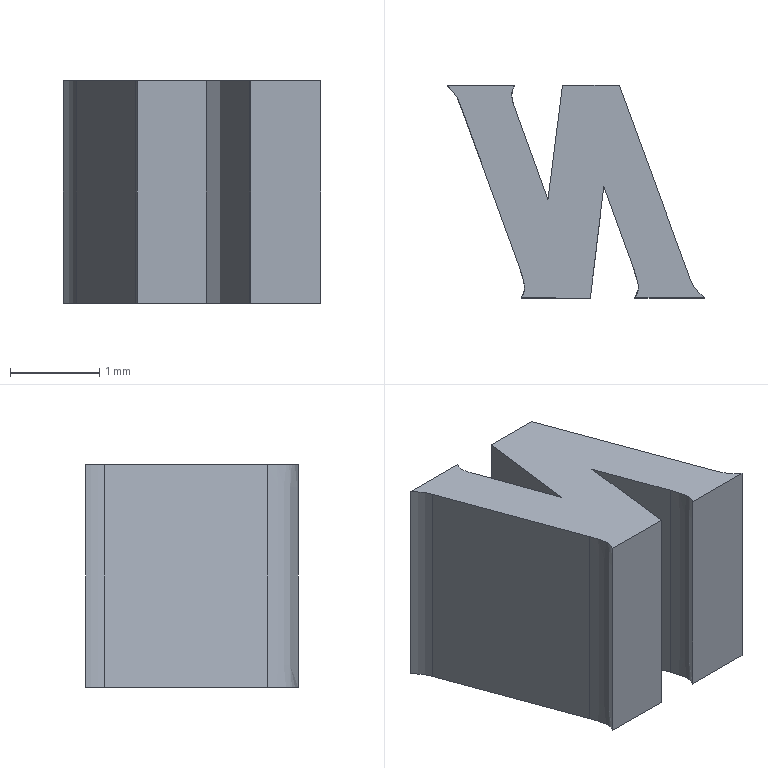Part | STEP file | lll_id1106_x_t | 1 solid | 18 faces | box 2.9 x 2.384 x 2.5 mm | volume 9.219 mm3 | plane 12 | cylinder 3 | other 3 | commonest cylinder face diameters 0.399 x1 0.832 x1 0.919 x1
STEP:
#1=CARTESIAN_POINT('',(389.276,-127.533,2.35));
#2=VERTEX_POINT('',#1);
#3=CARTESIAN_POINT('',(388.612,-125.708,2.35));
#4=VERTEX_POINT('',#3);
#5=CARTESIAN_POINT('',(389.276,-127.533,2.35));
#6=DIRECTION('',(-0.3422,0.9396,0.));
#7=VECTOR('',#6,1.);
#8=LINE('',#5,#7);
#9=EDGE_CURVE('',#2,#4,#8,.T.);
#10=ORIENTED_EDGE('',*,*,#9,.T.);
#11=CARTESIAN_POINT('',(388.612,-125.708,-0.15));
#12=VERTEX_POINT('',#11);
#13=CARTESIAN_POINT('',(388.612,-125.708,-0.15));
#14=DIRECTION('',(0.,0.,1.));
#15=VECTOR('',#14,1.);
#16=LINE('',#13,#15);
#17=EDGE_CURVE('',#12,#4,#16,.T.);
#18=ORIENTED_EDGE('',*,*,#17,.F.);
#19=CARTESIAN_POINT('',(389.276,-127.533,-0.15));
#20=VERTEX_POINT('',#19);
#21=CARTESIAN_POINT('',(389.276,-127.533,-0.15));
#22=DIRECTION('',(-0.3422,0.9396,0.));
#23=VECTOR('',#22,1.);
#24=LINE('',#21,#23);
#25=EDGE_CURVE('',#20,#12,#24,.T.);
#26=ORIENTED_EDGE('',*,*,#25,.F.);
#27=CARTESIAN_POINT('',(389.276,-127.533,-0.15));
#28=DIRECTION('',(0.,0.,1.));
#29=VECTOR('',#28,1.);
#30=LINE('',#27,#29);
#31=EDGE_CURVE('',#20,#2,#30,.T.);
#32=ORIENTED_EDGE('',*,*,#31,.T.);
#33=EDGE_LOOP('',(#10,#18,#26,#32));
#34=FACE_OUTER_BOUND('',#33,.T.);
#35=CARTESIAN_POINT('',(389.276,-127.533,-0.15));
#36=DIRECTION('',(0.9396,0.3422,0.));
#37=DIRECTION('',(0.3422,-0.9396,0.));
#38=AXIS2_PLACEMENT_3D('',#35,#36,#37);
#39=PLANE('',#38);
#40=ADVANCED_FACE('',(#34),#39,.F.);
#41=CARTESIAN_POINT('',(388.467,-125.495,2.35));
#42=VERTEX_POINT('',#41);
#43=CARTESIAN_POINT('',(388.176,-125.853,2.35));
#44=DIRECTION('',(0.,0.,1.));
#45=DIRECTION('',(-1.,0.,0.));
#46=AXIS2_PLACEMENT_3D('',#43,#44,#45);
#47=CIRCLE('',#46,0.4594);
#48=EDGE_CURVE('',#4,#42,#47,.T.);
#49=ORIENTED_EDGE('',*,*,#48,.T.);
#50=CARTESIAN_POINT('',(388.467,-125.495,-0.15));
#51=VERTEX_POINT('',#50);
#52=CARTESIAN_POINT('',(388.461,-125.492,-0.15));
#53=DIRECTION('',(0.,0.,1.));
#54=VECTOR('',#53,1.);
#55=LINE('',#52,#54);
#56=EDGE_CURVE('',#51,#42,#55,.T.);
#57=ORIENTED_EDGE('',*,*,#56,.F.);
#58=CARTESIAN_POINT('',(388.176,-125.853,-0.15));
#59=DIRECTION('',(0.,0.,1.));
#60=DIRECTION('',(-1.,0.,0.));
#61=AXIS2_PLACEMENT_3D('',#58,#59,#60);
#62=CIRCLE('',#61,0.4594);
#63=EDGE_CURVE('',#12,#51,#62,.T.);
#64=ORIENTED_EDGE('',*,*,#63,.F.);
#65=ORIENTED_EDGE('',*,*,#17,.T.);
#66=EDGE_LOOP('',(#49,#57,#64,#65));
#67=FACE_OUTER_BOUND('',#66,.T.);
#68=CARTESIAN_POINT('',(388.176,-125.853,-0.15));
#69=DIRECTION('',(0.,0.,1.));
#70=DIRECTION('',(1.,0.,0.));
#71=AXIS2_PLACEMENT_3D('',#68,#69,#70);
#72=CYLINDRICAL_SURFACE('',#71,0.4594);
#73=ADVANCED_FACE('',(#67),#72,.F.);
#74=CARTESIAN_POINT('',(389.22,-125.495,2.35));
#75=VERTEX_POINT('',#74);
#76=CARTESIAN_POINT('',(388.467,-125.492,2.35));
#77=DIRECTION('',(1.,0.,0.));
#78=VECTOR('',#77,1.);
#79=LINE('',#76,#78);
#80=EDGE_CURVE('',#42,#75,#79,.T.);
#81=ORIENTED_EDGE('',*,*,#80,.T.);
#82=CARTESIAN_POINT('',(389.22,-125.495,-0.15));
#83=VERTEX_POINT('',#82);
#84=CARTESIAN_POINT('',(389.224,-125.492,-0.15));
#85=DIRECTION('',(0.,0.,1.));
#86=VECTOR('',#85,1.);
#87=LINE('',#84,#86);
#88=EDGE_CURVE('',#83,#75,#87,.T.);
#89=ORIENTED_EDGE('',*,*,#88,.F.);
#90=CARTESIAN_POINT('',(388.467,-125.492,-0.15));
#91=DIRECTION('',(1.,0.,0.));
#92=VECTOR('',#91,1.);
#93=LINE('',#90,#92);
#94=EDGE_CURVE('',#51,#83,#93,.T.);
#95=ORIENTED_EDGE('',*,*,#94,.F.);
#96=ORIENTED_EDGE('',*,*,#56,.T.);
#97=EDGE_LOOP('',(#81,#89,#95,#96));
#98=FACE_OUTER_BOUND('',#97,.T.);
#99=CARTESIAN_POINT('',(388.467,-125.492,-0.15));
#100=DIRECTION('',(0.,-1.,0.));
#101=DIRECTION('',(0.,0.,-1.));
#102=AXIS2_PLACEMENT_3D('',#99,#100,#101);
#103=PLANE('',#102);
#104=ADVANCED_FACE('',(#98),#103,.F.);
#105=CARTESIAN_POINT('',(389.2,-125.536,2.35));
#106=VERTEX_POINT('',#105);
#107=CARTESIAN_POINT('',(389.221,-125.497,2.35));
#108=CARTESIAN_POINT('',(389.212,-125.509,2.35));
#109=CARTESIAN_POINT('',(389.205,-125.522,2.35));
#110=CARTESIAN_POINT('',(389.2,-125.536,2.35));
#111=(BOUNDED_CURVE()B_SPLINE_CURVE(3,(#107,#108,#109,#110),.UNSPECIFIED.,.F.,.F.)B_SPLINE_CURVE_WITH_KNOTS((4,4),(0.,1.),.UNSPECIFIED.)CURVE()GEOMETRIC_REPRESENTATION_ITEM()RATIONAL_B_SPLINE_CURVE((0.5015,0.4995,0.4995,0.5015))REPRESENTATION_ITEM(''));
#112=EDGE_CURVE('',#75,#106,#111,.T.);
#113=ORIENTED_EDGE('',*,*,#112,.T.);
#114=CARTESIAN_POINT('',(389.2,-125.536,-0.15));
#115=VERTEX_POINT('',#114);
#116=CARTESIAN_POINT('',(389.2,-125.536,-0.15));
#117=DIRECTION('',(0.,0.,1.));
#118=VECTOR('',#117,1.);
#119=LINE('',#116,#118);
#120=EDGE_CURVE('',#115,#106,#119,.T.);
#121=ORIENTED_EDGE('',*,*,#120,.F.);
#122=CARTESIAN_POINT('',(389.221,-125.497,-0.15));
#123=CARTESIAN_POINT('',(389.212,-125.509,-0.15));
#124=CARTESIAN_POINT('',(389.205,-125.522,-0.15));
#125=CARTESIAN_POINT('',(389.2,-125.536,-0.15));
#126=(BOUNDED_CURVE()B_SPLINE_CURVE(3,(#122,#123,#124,#125),.UNSPECIFIED.,.F.,.F.)B_SPLINE_CURVE_WITH_KNOTS((4,4),(0.,1.),.UNSPECIFIED.)CURVE()GEOMETRIC_REPRESENTATION_ITEM()RATIONAL_B_SPLINE_CURVE((0.5015,0.4995,0.4995,0.5015))REPRESENTATION_ITEM(''));
#127=EDGE_CURVE('',#83,#115,#126,.T.);
#128=ORIENTED_EDGE('',*,*,#127,.F.);
#129=ORIENTED_EDGE('',*,*,#88,.T.);
#130=EDGE_LOOP('',(#113,#121,#128,#129));
#131=FACE_OUTER_BOUND('',#130,.T.);
#132=CARTESIAN_POINT('',(389.385,-125.611,-0.15));
#133=DIRECTION('',(0.,0.,1.));
#134=DIRECTION('',(1.,0.,0.));
#135=AXIS2_PLACEMENT_3D('',#132,#133,#134);
#136=CYLINDRICAL_SURFACE('',#135,0.1994);
#137=ADVANCED_FACE('',(#131),#136,.F.);
#138=CARTESIAN_POINT('',(389.21,-125.704,2.35));
#139=VERTEX_POINT('',#138);
#140=CARTESIAN_POINT('',(389.2,-125.536,2.35));
#141=CARTESIAN_POINT('',(389.194,-125.552,2.35));
#142=CARTESIAN_POINT('',(389.19,-125.568,2.35));
#143=CARTESIAN_POINT('',(389.188,-125.592,2.35));
#144=CARTESIAN_POINT('',(389.188,-125.599,2.35));
#145=CARTESIAN_POINT('',(389.189,-125.617,2.35));
#146=CARTESIAN_POINT('',(389.19,-125.628,2.35));
#147=CARTESIAN_POINT('',(389.194,-125.65,2.35));
#148=CARTESIAN_POINT('',(389.196,-125.661,2.35));
#149=CARTESIAN_POINT('',(389.202,-125.683,2.35));
#150=CARTESIAN_POINT('',(389.206,-125.693,2.35));
#151=CARTESIAN_POINT('',(389.21,-125.704,2.35));
#152=(BOUNDED_CURVE()B_SPLINE_CURVE(3,(#140,#141,#142,#143,#144,#145,#146,#147,#148,#149,#150,#151),.UNSPECIFIED.,.F.,.F.)B_SPLINE_CURVE_WITH_KNOTS((4,2,2,2,2,4),(0.,0.2962,0.4138,0.6091,0.8048,1.),.UNSPECIFIED.)CURVE()GEOMETRIC_REPRESENTATION_ITEM()RATIONAL_B_SPLINE_CURVE((0.5015,0.4975,0.4975,0.5011,0.5011,0.5008,0.5008,0.5011,0.5011,0.5013,0.5013,0.5015))REPRESENTATION_ITEM(''));
#153=EDGE_CURVE('',#106,#139,#152,.T.);
#154=ORIENTED_EDGE('',*,*,#153,.T.);
#155=CARTESIAN_POINT('',(389.21,-125.704,-0.15));
#156=VERTEX_POINT('',#155);
#157=CARTESIAN_POINT('',(389.21,-125.704,-0.15));
#158=DIRECTION('',(0.,0.,1.));
#159=VECTOR('',#158,1.);
#160=LINE('',#157,#159);
#161=EDGE_CURVE('',#156,#139,#160,.T.);
#162=ORIENTED_EDGE('',*,*,#161,.F.);
#163=CARTESIAN_POINT('',(389.2,-125.536,-0.15));
#164=CARTESIAN_POINT('',(389.194,-125.552,-0.15));
#165=CARTESIAN_POINT('',(389.19,-125.568,-0.15));
#166=CARTESIAN_POINT('',(389.188,-125.592,-0.15));
#167=CARTESIAN_POINT('',(389.188,-125.599,-0.15));
#168=CARTESIAN_POINT('',(389.189,-125.617,-0.15));
#169=CARTESIAN_POINT('',(389.19,-125.628,-0.15));
#170=CARTESIAN_POINT('',(389.194,-125.65,-0.15));
#171=CARTESIAN_POINT('',(389.196,-125.661,-0.15));
#172=CARTESIAN_POINT('',(389.202,-125.683,-0.15));
#173=CARTESIAN_POINT('',(389.206,-125.693,-0.15));
#174=CARTESIAN_POINT('',(389.21,-125.704,-0.15));
#175=(BOUNDED_CURVE()B_SPLINE_CURVE(3,(#163,#164,#165,#166,#167,#168,#169,#170,#171,#172,#173,#174),.UNSPECIFIED.,.F.,.F.)B_SPLINE_CURVE_WITH_KNOTS((4,2,2,2,2,4),(0.,0.2962,0.4138,0.6091,0.8048,1.),.UNSPECIFIED.)CURVE()GEOMETRIC_REPRESENTATION_ITEM()RATIONAL_B_SPLINE_CURVE((0.5015,0.4975,0.4975,0.5011,0.5011,0.5008,0.5008,0.5011,0.5011,0.5013,0.5013,0.5015))REPRESENTATION_ITEM(''));
#176=EDGE_CURVE('',#115,#156,#175,.T.);
#177=ORIENTED_EDGE('',*,*,#176,.F.);
#178=ORIENTED_EDGE('',*,*,#120,.T.);
#179=EDGE_LOOP('',(#154,#162,#177,#178));
#180=FACE_OUTER_BOUND('',#179,.T.);
#181=CARTESIAN_POINT('',(389.2,-125.536,-0.15));
#182=CARTESIAN_POINT('',(389.194,-125.552,-0.15));
#183=CARTESIAN_POINT('',(389.19,-125.568,-0.15));
#184=CARTESIAN_POINT('',(389.188,-125.592,-0.15));
#185=CARTESIAN_POINT('',(389.188,-125.599,-0.15));
#186=CARTESIAN_POINT('',(389.189,-125.617,-0.15));
#187=CARTESIAN_POINT('',(389.19,-125.628,-0.15));
#188=CARTESIAN_POINT('',(389.194,-125.65,-0.15));
#189=CARTESIAN_POINT('',(389.196,-125.661,-0.15));
#190=CARTESIAN_POINT('',(389.202,-125.683,-0.15));
#191=CARTESIAN_POINT('',(389.206,-125.693,-0.15));
#192=CARTESIAN_POINT('',(389.21,-125.704,-0.15));
#193=(BOUNDED_CURVE()B_SPLINE_CURVE(3,(#181,#182,#183,#184,#185,#186,#187,#188,#189,#190,#191,#192),.UNSPECIFIED.,.F.,.F.)B_SPLINE_CURVE_WITH_KNOTS((4,2,2,2,2,4),(0.,0.2962,0.4138,0.6091,0.8048,1.),.UNSPECIFIED.)CURVE()GEOMETRIC_REPRESENTATION_ITEM()RATIONAL_B_SPLINE_CURVE((0.5015,0.4975,0.4975,0.5011,0.5011,0.5008,0.5008,0.5011,0.5011,0.5013,0.5013,0.5015))REPRESENTATION_ITEM(''));
#194=DIRECTION('',(0.,0.,1.));
#195=VECTOR('',#194,1.);
#196=SURFACE_OF_LINEAR_EXTRUSION('',#193,#195);
#197=ADVANCED_FACE('',(#180),#196,.F.);
#198=CARTESIAN_POINT('',(389.595,-126.775,2.35));
#199=VERTEX_POINT('',#198);
#200=CARTESIAN_POINT('',(389.21,-125.704,2.35));
#201=DIRECTION('',(0.3387,-0.9409,0.));
#202=VECTOR('',#201,1.);
#203=LINE('',#200,#202);
#204=EDGE_CURVE('',#139,#199,#203,.T.);
#205=ORIENTED_EDGE('',*,*,#204,.T.);
#206=CARTESIAN_POINT('',(389.595,-126.775,-0.15));
#207=VERTEX_POINT('',#206);
#208=CARTESIAN_POINT('',(389.595,-126.775,-0.15));
#209=DIRECTION('',(0.,0.,1.));
#210=VECTOR('',#209,1.);
#211=LINE('',#208,#210);
#212=EDGE_CURVE('',#207,#199,#211,.T.);
#213=ORIENTED_EDGE('',*,*,#212,.F.);
#214=CARTESIAN_POINT('',(389.21,-125.704,-0.15));
#215=DIRECTION('',(0.3387,-0.9409,0.));
#216=VECTOR('',#215,1.);
#217=LINE('',#214,#216);
#218=EDGE_CURVE('',#156,#207,#217,.T.);
#219=ORIENTED_EDGE('',*,*,#218,.F.);
#220=ORIENTED_EDGE('',*,*,#161,.T.);
#221=EDGE_LOOP('',(#205,#213,#219,#220));
#222=FACE_OUTER_BOUND('',#221,.T.);
#223=CARTESIAN_POINT('',(389.21,-125.704,-0.15));
#224=DIRECTION('',(-0.9409,-0.3387,0.));
#225=DIRECTION('',(-0.3387,0.9409,0.));
#226=AXIS2_PLACEMENT_3D('',#223,#224,#225);
#227=PLANE('',#226);
#228=ADVANCED_FACE('',(#222),#227,.F.);
#229=CARTESIAN_POINT('',(389.758,-125.492,2.35));
#230=VERTEX_POINT('',#229);
#231=CARTESIAN_POINT('',(389.595,-126.775,2.35));
#232=DIRECTION('',(0.1257,0.9921,0.));
#233=VECTOR('',#232,1.);
#234=LINE('',#231,#233);
#235=EDGE_CURVE('',#199,#230,#234,.T.);
#236=ORIENTED_EDGE('',*,*,#235,.T.);
#237=CARTESIAN_POINT('',(389.758,-125.492,-0.15));
#238=VERTEX_POINT('',#237);
#239=CARTESIAN_POINT('',(389.758,-125.492,-0.15));
#240=DIRECTION('',(0.,0.,1.));
#241=VECTOR('',#240,1.);
#242=LINE('',#239,#241);
#243=EDGE_CURVE('',#238,#230,#242,.T.);
#244=ORIENTED_EDGE('',*,*,#243,.F.);
#245=CARTESIAN_POINT('',(389.595,-126.775,-0.15));
#246=DIRECTION('',(0.1257,0.9921,0.));
#247=VECTOR('',#246,1.);
#248=LINE('',#245,#247);
#249=EDGE_CURVE('',#207,#238,#248,.T.);
#250=ORIENTED_EDGE('',*,*,#249,.F.);
#251=ORIENTED_EDGE('',*,*,#212,.T.);
#252=EDGE_LOOP('',(#236,#244,#250,#251));
#253=FACE_OUTER_BOUND('',#252,.T.);
#254=CARTESIAN_POINT('',(389.595,-126.775,-0.15));
#255=DIRECTION('',(0.9921,-0.1257,0.));
#256=DIRECTION('',(-0.1257,-0.9921,0.));
#257=AXIS2_PLACEMENT_3D('',#254,#255,#256);
#258=PLANE('',#257);
#259=ADVANCED_FACE('',(#253),#258,.F.);
#260=CARTESIAN_POINT('',(390.396,-125.492,2.35));
#261=VERTEX_POINT('',#260);
#262=CARTESIAN_POINT('',(389.758,-125.492,2.35));
#263=DIRECTION('',(1.,0.,0.));
#264=VECTOR('',#263,1.);
#265=LINE('',#262,#264);
#266=EDGE_CURVE('',#230,#261,#265,.T.);
#267=ORIENTED_EDGE('',*,*,#266,.T.);
#268=CARTESIAN_POINT('',(390.396,-125.492,-0.15));
#269=VERTEX_POINT('',#268);
#270=CARTESIAN_POINT('',(390.396,-125.492,-0.15));
#271=DIRECTION('',(0.,0.,1.));
#272=VECTOR('',#271,1.);
#273=LINE('',#270,#272);
#274=EDGE_CURVE('',#269,#261,#273,.T.);
#275=ORIENTED_EDGE('',*,*,#274,.F.);
#276=CARTESIAN_POINT('',(389.758,-125.492,-0.15));
#277=DIRECTION('',(1.,0.,0.));
#278=VECTOR('',#277,1.);
#279=LINE('',#276,#278);
#280=EDGE_CURVE('',#238,#269,#279,.T.);
#281=ORIENTED_EDGE('',*,*,#280,.F.);
#282=ORIENTED_EDGE('',*,*,#243,.T.);
#283=EDGE_LOOP('',(#267,#275,#281,#282));
#284=FACE_OUTER_BOUND('',#283,.T.);
#285=CARTESIAN_POINT('',(389.758,-125.492,-0.15));
#286=DIRECTION('',(0.,-1.,0.));
#287=DIRECTION('',(0.,0.,-1.));
#288=AXIS2_PLACEMENT_3D('',#285,#286,#287);
#289=PLANE('',#288);
#290=ADVANCED_FACE('',(#284),#289,.F.);
#291=CARTESIAN_POINT('',(391.191,-127.665,2.35));
#292=VERTEX_POINT('',#291);
#293=CARTESIAN_POINT('',(390.396,-125.492,2.35));
#294=DIRECTION('',(0.3436,-0.9391,0.));
#295=VECTOR('',#294,1.);
#296=LINE('',#293,#295);
#297=EDGE_CURVE('',#261,#292,#296,.T.);
#298=ORIENTED_EDGE('',*,*,#297,.T.);
#299=CARTESIAN_POINT('',(391.191,-127.665,-0.15));
#300=VERTEX_POINT('',#299);
#301=CARTESIAN_POINT('',(391.191,-127.665,-0.15));
#302=DIRECTION('',(0.,0.,1.));
#303=VECTOR('',#302,1.);
#304=LINE('',#301,#303);
#305=EDGE_CURVE('',#300,#292,#304,.T.);
#306=ORIENTED_EDGE('',*,*,#305,.F.);
#307=CARTESIAN_POINT('',(390.396,-125.492,-0.15));
#308=DIRECTION('',(0.3436,-0.9391,0.));
#309=VECTOR('',#308,1.);
#310=LINE('',#307,#309);
#311=EDGE_CURVE('',#269,#300,#310,.T.);
#312=ORIENTED_EDGE('',*,*,#311,.F.);
#313=ORIENTED_EDGE('',*,*,#274,.T.);
#314=EDGE_LOOP('',(#298,#306,#312,#313));
#315=FACE_OUTER_BOUND('',#314,.T.);
#316=CARTESIAN_POINT('',(390.396,-125.492,-0.15));
#317=DIRECTION('',(-0.9391,-0.3436,0.));
#318=DIRECTION('',(-0.3436,0.9391,0.));
#319=AXIS2_PLACEMENT_3D('',#316,#317,#318);
#320=PLANE('',#319);
#321=ADVANCED_FACE('',(#315),#320,.F.);
#322=CARTESIAN_POINT('',(391.352,-127.874,2.35));
#323=VERTEX_POINT('',#322);
#324=CARTESIAN_POINT('',(391.583,-127.525,2.35));
#325=DIRECTION('',(0.,0.,1.));
#326=DIRECTION('',(-1.,0.,0.));
#327=AXIS2_PLACEMENT_3D('',#324,#325,#326);
#328=CIRCLE('',#327,0.4162);
#329=EDGE_CURVE('',#292,#323,#328,.T.);
#330=ORIENTED_EDGE('',*,*,#329,.T.);
#331=CARTESIAN_POINT('',(391.352,-127.874,-0.15));
#332=VERTEX_POINT('',#331);
#333=CARTESIAN_POINT('',(391.361,-127.876,-0.15));
#334=DIRECTION('',(0.,0.,1.));
#335=VECTOR('',#334,1.);
#336=LINE('',#333,#335);
#337=EDGE_CURVE('',#332,#323,#336,.T.);
#338=ORIENTED_EDGE('',*,*,#337,.F.);
#339=CARTESIAN_POINT('',(391.583,-127.525,-0.15));
#340=DIRECTION('',(0.,0.,1.));
#341=DIRECTION('',(-1.,0.,0.));
#342=AXIS2_PLACEMENT_3D('',#339,#340,#341);
#343=CIRCLE('',#342,0.4162);
#344=EDGE_CURVE('',#300,#332,#343,.T.);
#345=ORIENTED_EDGE('',*,*,#344,.F.);
#346=ORIENTED_EDGE('',*,*,#305,.T.);
#347=EDGE_LOOP('',(#330,#338,#345,#346));
#348=FACE_OUTER_BOUND('',#347,.T.);
#349=CARTESIAN_POINT('',(391.583,-127.525,-0.15));
#350=DIRECTION('',(0.,0.,1.));
#351=DIRECTION('',(1.,0.,0.));
#352=AXIS2_PLACEMENT_3D('',#349,#350,#351);
#353=CYLINDRICAL_SURFACE('',#352,0.4162);
#354=ADVANCED_FACE('',(#348),#353,.F.);
#355=CARTESIAN_POINT('',(390.569,-127.874,2.35));
#356=VERTEX_POINT('',#355);
#357=CARTESIAN_POINT('',(391.352,-127.876,2.35));
#358=DIRECTION('',(-1.,0.,0.));
#359=VECTOR('',#358,1.);
#360=LINE('',#357,#359);
#361=EDGE_CURVE('',#323,#356,#360,.T.);
#362=ORIENTED_EDGE('',*,*,#361,.T.);
#363=CARTESIAN_POINT('',(390.569,-127.874,-0.15));
#364=VERTEX_POINT('',#363);
#365=CARTESIAN_POINT('',(390.565,-127.876,-0.15));
#366=DIRECTION('',(0.,0.,1.));
#367=VECTOR('',#366,1.);
#368=LINE('',#365,#367);
#369=EDGE_CURVE('',#364,#356,#368,.T.);
#370=ORIENTED_EDGE('',*,*,#369,.F.);
#371=CARTESIAN_POINT('',(391.352,-127.876,-0.15));
#372=DIRECTION('',(-1.,0.,0.));
#373=VECTOR('',#372,1.);
#374=LINE('',#371,#373);
#375=EDGE_CURVE('',#332,#364,#374,.T.);
#376=ORIENTED_EDGE('',*,*,#375,.F.);
#377=ORIENTED_EDGE('',*,*,#337,.T.);
#378=EDGE_LOOP('',(#362,#370,#376,#377));
#379=FACE_OUTER_BOUND('',#378,.T.);
#380=CARTESIAN_POINT('',(391.352,-127.876,-0.15));
#381=DIRECTION('',(0.,1.,0.));
#382=DIRECTION('',(0.,0.,1.));
#383=AXIS2_PLACEMENT_3D('',#380,#381,#382);
#384=PLANE('',#383);
#385=ADVANCED_FACE('',(#379),#384,.F.);
#386=CARTESIAN_POINT('',(390.552,-127.533,2.35));
#387=VERTEX_POINT('',#386);
#388=CARTESIAN_POINT('',(390.569,-127.871,2.35));
#389=CARTESIAN_POINT('',(390.572,-127.868,2.35));
#390=CARTESIAN_POINT('',(390.574,-127.865,2.35));
#391=CARTESIAN_POINT('',(390.594,-127.838,2.35));
#392=CARTESIAN_POINT('',(390.605,-127.81,2.35));
#393=CARTESIAN_POINT('',(390.609,-127.768,2.35));
#394=CARTESIAN_POINT('',(390.609,-127.755,2.35));
#395=CARTESIAN_POINT('',(390.607,-127.732,2.35));
#396=CARTESIAN_POINT('',(390.606,-127.723,2.35));
#397=CARTESIAN_POINT('',(390.603,-127.703,2.35));
#398=CARTESIAN_POINT('',(390.601,-127.692,2.35));
#399=CARTESIAN_POINT('',(390.595,-127.671,2.35));
#400=CARTESIAN_POINT('',(390.593,-127.66,2.35));
#401=CARTESIAN_POINT('',(390.584,-127.631,2.35));
#402=CARTESIAN_POINT('',(390.579,-127.614,2.35));
#403=CARTESIAN_POINT('',(390.567,-127.575,2.35));
#404=CARTESIAN_POINT('',(390.56,-127.554,2.35));
#405=CARTESIAN_POINT('',(390.552,-127.533,2.35));
#406=(BOUNDED_CURVE()B_SPLINE_CURVE(3,(#388,#389,#390,#391,#392,#393,#394,#395,#396,#397,#398,#399,#400,#401,#402,#403,#404,#405),.UNSPECIFIED.,.F.,.F.)B_SPLINE_CURVE_WITH_KNOTS((4,2,2,2,2,2,2,2,4),(0.,0.03221,0.285,0.3941,0.4717,0.5649,0.6583,0.8136,1.),.UNSPECIFIED.)CURVE()GEOMETRIC_REPRESENTATION_ITEM()RATIONAL_B_SPLINE_CURVE((0.5001,0.5,0.5,0.4872,0.4872,0.4988,0.4988,0.4998,0.4998,0.4998,0.4998,0.5,0.5,0.5,0.5,0.5,0.5,0.5001))REPRESENTATION_ITEM(''));
#407=EDGE_CURVE('',#356,#387,#406,.T.);
#408=ORIENTED_EDGE('',*,*,#407,.T.);
#409=CARTESIAN_POINT('',(390.552,-127.533,-0.15));
#410=VERTEX_POINT('',#409);
#411=CARTESIAN_POINT('',(390.552,-127.533,-0.15));
#412=DIRECTION('',(0.,0.,1.));
#413=VECTOR('',#412,1.);
#414=LINE('',#411,#413);
#415=EDGE_CURVE('',#410,#387,#414,.T.);
#416=ORIENTED_EDGE('',*,*,#415,.F.);
#417=CARTESIAN_POINT('',(390.567,-127.874,-0.15));
#418=CARTESIAN_POINT('',(390.568,-127.873,-0.15));
#419=CARTESIAN_POINT('',(390.568,-127.872,-0.15));
#420=CARTESIAN_POINT('',(390.572,-127.868,-0.15));
#421=CARTESIAN_POINT('',(390.574,-127.865,-0.15));
#422=CARTESIAN_POINT('',(390.594,-127.838,-0.15));
#423=CARTESIAN_POINT('',(390.605,-127.81,-0.15));
#424=CARTESIAN_POINT('',(390.609,-127.768,-0.15));
#425=CARTESIAN_POINT('',(390.609,-127.755,-0.15));
#426=CARTESIAN_POINT('',(390.607,-127.732,-0.15));
#427=CARTESIAN_POINT('',(390.606,-127.723,-0.15));
#428=CARTESIAN_POINT('',(390.603,-127.703,-0.15));
#429=CARTESIAN_POINT('',(390.601,-127.692,-0.15));
#430=CARTESIAN_POINT('',(390.595,-127.671,-0.15));
#431=CARTESIAN_POINT('',(390.593,-127.66,-0.15));
#432=CARTESIAN_POINT('',(390.584,-127.631,-0.15));
#433=CARTESIAN_POINT('',(390.579,-127.614,-0.15));
#434=CARTESIAN_POINT('',(390.567,-127.575,-0.15));
#435=CARTESIAN_POINT('',(390.56,-127.554,-0.15));
#436=CARTESIAN_POINT('',(390.552,-127.533,-0.15));
#437=(BOUNDED_CURVE()B_SPLINE_CURVE(3,(#417,#418,#419,#420,#421,#422,#423,#424,#425,#426,#427,#428,#429,#430,#431,#432,#433,#434,#435,#436),.UNSPECIFIED.,.F.,.F.)B_SPLINE_CURVE_WITH_KNOTS((4,2,2,2,2,2,2,2,2,4),(0.,0.009901,0.04179,0.2921,0.4001,0.4769,0.5692,0.6617,0.8154,1.),.UNSPECIFIED.)CURVE()GEOMETRIC_REPRESENTATION_ITEM()RATIONAL_B_SPLINE_CURVE((0.5001,0.5001,0.5001,0.5,0.5,0.4872,0.4872,0.4988,0.4988,0.4998,0.4998,0.4998,0.4998,0.5,0.5,0.5,0.5,0.5,0.5,0.5001))REPRESENTATION_ITEM(''));
#438=EDGE_CURVE('',#364,#410,#437,.T.);
#439=ORIENTED_EDGE('',*,*,#438,.F.);
#440=ORIENTED_EDGE('',*,*,#369,.T.);
#441=EDGE_LOOP('',(#408,#416,#439,#440));
#442=FACE_OUTER_BOUND('',#441,.T.);
#443=CARTESIAN_POINT('',(390.565,-127.876,-0.15));
#444=CARTESIAN_POINT('',(390.565,-127.875,-0.15));
#445=CARTESIAN_POINT('',(390.566,-127.875,-0.15));
#446=CARTESIAN_POINT('',(390.568,-127.873,-0.15));
#447=CARTESIAN_POINT('',(390.568,-127.872,-0.15));
#448=CARTESIAN_POINT('',(390.572,-127.868,-0.15));
#449=CARTESIAN_POINT('',(390.574,-127.865,-0.15));
#450=CARTESIAN_POINT('',(390.594,-127.838,-0.15));
#451=CARTESIAN_POINT('',(390.605,-127.81,-0.15));
#452=CARTESIAN_POINT('',(390.609,-127.768,-0.15));
#453=CARTESIAN_POINT('',(390.609,-127.755,-0.15));
#454=CARTESIAN_POINT('',(390.607,-127.732,-0.15));
#455=CARTESIAN_POINT('',(390.606,-127.723,-0.15));
#456=CARTESIAN_POINT('',(390.603,-127.703,-0.15));
#457=CARTESIAN_POINT('',(390.601,-127.692,-0.15));
#458=CARTESIAN_POINT('',(390.595,-127.671,-0.15));
#459=CARTESIAN_POINT('',(390.593,-127.66,-0.15));
#460=CARTESIAN_POINT('',(390.584,-127.631,-0.15));
#461=CARTESIAN_POINT('',(390.579,-127.614,-0.15));
#462=CARTESIAN_POINT('',(390.567,-127.575,-0.15));
#463=CARTESIAN_POINT('',(390.56,-127.554,-0.15));
#464=CARTESIAN_POINT('',(390.552,-127.533,-0.15));
#465=(BOUNDED_CURVE()B_SPLINE_CURVE(3,(#443,#444,#445,#446,#447,#448,#449,#450,#451,#452,#453,#454,#455,#456,#457,#458,#459,#460,#461,#462,#463,#464),.UNSPECIFIED.,.F.,.F.)B_SPLINE_CURVE_WITH_KNOTS((4,2,2,2,2,2,2,2,2,2,4),(0.,0.01012,0.01992,0.05149,0.2993,0.4062,0.4822,0.5736,0.6651,0.8173,1.),.UNSPECIFIED.)CURVE()GEOMETRIC_REPRESENTATION_ITEM()RATIONAL_B_SPLINE_CURVE((0.5001,0.5001,0.5001,0.5001,0.5001,0.5,0.5,0.4872,0.4872,0.4988,0.4988,0.4998,0.4998,0.4998,0.4998,0.5,0.5,0.5,0.5,0.5,0.5,0.5001))REPRESENTATION_ITEM(''));
#466=DIRECTION('',(0.,0.,1.));
#467=VECTOR('',#466,1.);
#468=SURFACE_OF_LINEAR_EXTRUSION('',#465,#467);
#469=ADVANCED_FACE('',(#442),#468,.F.);
#470=CARTESIAN_POINT('',(390.221,-126.625,2.35));
#471=VERTEX_POINT('',#470);
#472=CARTESIAN_POINT('',(390.552,-127.533,2.35));
#473=DIRECTION('',(-0.3421,0.9397,0.));
#474=VECTOR('',#473,1.);
#475=LINE('',#472,#474);
#476=EDGE_CURVE('',#387,#471,#475,.T.);
#477=ORIENTED_EDGE('',*,*,#476,.T.);
#478=CARTESIAN_POINT('',(390.221,-126.625,-0.15));
#479=VERTEX_POINT('',#478);
#480=CARTESIAN_POINT('',(390.221,-126.625,-0.15));
#481=DIRECTION('',(0.,0.,1.));
#482=VECTOR('',#481,1.);
#483=LINE('',#480,#482);
#484=EDGE_CURVE('',#479,#471,#483,.T.);
#485=ORIENTED_EDGE('',*,*,#484,.F.);
#486=CARTESIAN_POINT('',(390.552,-127.533,-0.15));
#487=DIRECTION('',(-0.3421,0.9397,0.));
#488=VECTOR('',#487,1.);
#489=LINE('',#486,#488);
#490=EDGE_CURVE('',#410,#479,#489,.T.);
#491=ORIENTED_EDGE('',*,*,#490,.F.);
#492=ORIENTED_EDGE('',*,*,#415,.T.);
#493=EDGE_LOOP('',(#477,#485,#491,#492));
#494=FACE_OUTER_BOUND('',#493,.T.);
#495=CARTESIAN_POINT('',(390.552,-127.533,-0.15));
#496=DIRECTION('',(0.9397,0.3421,0.));
#497=DIRECTION('',(0.3421,-0.9397,0.));
#498=AXIS2_PLACEMENT_3D('',#495,#496,#497);
#499=PLANE('',#498);
#500=ADVANCED_FACE('',(#494),#499,.F.);
#501=CARTESIAN_POINT('',(390.07,-127.876,2.35));
#502=VERTEX_POINT('',#501);
#503=CARTESIAN_POINT('',(390.221,-126.625,2.35));
#504=DIRECTION('',(-0.1198,-0.9928,0.));
#505=VECTOR('',#504,1.);
#506=LINE('',#503,#505);
#507=EDGE_CURVE('',#471,#502,#506,.T.);
#508=ORIENTED_EDGE('',*,*,#507,.T.);
#509=CARTESIAN_POINT('',(390.07,-127.876,-0.15));
#510=VERTEX_POINT('',#509);
#511=CARTESIAN_POINT('',(390.07,-127.876,-0.15));
#512=DIRECTION('',(0.,0.,1.));
#513=VECTOR('',#512,1.);
#514=LINE('',#511,#513);
#515=EDGE_CURVE('',#510,#502,#514,.T.);
#516=ORIENTED_EDGE('',*,*,#515,.F.);
#517=CARTESIAN_POINT('',(390.221,-126.625,-0.15));
#518=DIRECTION('',(-0.1198,-0.9928,0.));
#519=VECTOR('',#518,1.);
#520=LINE('',#517,#519);
#521=EDGE_CURVE('',#479,#510,#520,.T.);
#522=ORIENTED_EDGE('',*,*,#521,.F.);
#523=ORIENTED_EDGE('',*,*,#484,.T.);
#524=EDGE_LOOP('',(#508,#516,#522,#523));
#525=FACE_OUTER_BOUND('',#524,.T.);
#526=CARTESIAN_POINT('',(390.221,-126.625,-0.15));
#527=DIRECTION('',(-0.9928,0.1198,0.));
#528=DIRECTION('',(0.1198,0.9928,0.));
#529=AXIS2_PLACEMENT_3D('',#526,#527,#528);
#530=PLANE('',#529);
#531=ADVANCED_FACE('',(#525),#530,.F.);
#532=CARTESIAN_POINT('',(389.294,-127.874,2.35));
#533=VERTEX_POINT('',#532);
#534=CARTESIAN_POINT('',(390.07,-127.876,2.35));
#535=DIRECTION('',(-1.,0.,0.));
#536=VECTOR('',#535,1.);
#537=LINE('',#534,#536);
#538=EDGE_CURVE('',#502,#533,#537,.T.);
#539=ORIENTED_EDGE('',*,*,#538,.T.);
#540=CARTESIAN_POINT('',(389.294,-127.874,-0.15));
#541=VERTEX_POINT('',#540);
#542=CARTESIAN_POINT('',(389.289,-127.876,-0.15));
#543=DIRECTION('',(0.,0.,1.));
#544=VECTOR('',#543,1.);
#545=LINE('',#542,#544);
#546=EDGE_CURVE('',#541,#533,#545,.T.);
#547=ORIENTED_EDGE('',*,*,#546,.F.);
#548=CARTESIAN_POINT('',(390.07,-127.876,-0.15));
#549=DIRECTION('',(-1.,0.,0.));
#550=VECTOR('',#549,1.);
#551=LINE('',#548,#550);
#552=EDGE_CURVE('',#510,#541,#551,.T.);
#553=ORIENTED_EDGE('',*,*,#552,.F.);
#554=ORIENTED_EDGE('',*,*,#515,.T.);
#555=EDGE_LOOP('',(#539,#547,#553,#554));
#556=FACE_OUTER_BOUND('',#555,.T.);
#557=CARTESIAN_POINT('',(390.07,-127.876,-0.15));
#558=DIRECTION('',(0.,1.,0.));
#559=DIRECTION('',(0.,0.,1.));
#560=AXIS2_PLACEMENT_3D('',#557,#558,#559);
#561=PLANE('',#560);
#562=ADVANCED_FACE('',(#556),#561,.F.);
#563=CARTESIAN_POINT('',(389.294,-127.871,2.35));
#564=CARTESIAN_POINT('',(389.296,-127.868,2.35));
#565=CARTESIAN_POINT('',(389.298,-127.865,2.35));
#566=CARTESIAN_POINT('',(389.318,-127.84,2.35));
#567=CARTESIAN_POINT('',(389.328,-127.814,2.35));
#568=CARTESIAN_POINT('',(389.333,-127.773,2.35));
#569=CARTESIAN_POINT('',(389.333,-127.76,2.35));
#570=CARTESIAN_POINT('',(389.332,-127.736,2.35));
#571=CARTESIAN_POINT('',(389.331,-127.725,2.35));
#572=CARTESIAN_POINT('',(389.327,-127.703,2.35));
#573=CARTESIAN_POINT('',(389.325,-127.692,2.35));
#574=CARTESIAN_POINT('',(389.32,-127.671,2.35));
#575=CARTESIAN_POINT('',(389.317,-127.66,2.35));
#576=CARTESIAN_POINT('',(389.309,-127.631,2.35));
#577=CARTESIAN_POINT('',(389.303,-127.614,2.35));
#578=CARTESIAN_POINT('',(389.291,-127.575,2.35));
#579=CARTESIAN_POINT('',(389.284,-127.554,2.35));
#580=CARTESIAN_POINT('',(389.276,-127.533,2.35));
#581=(BOUNDED_CURVE()B_SPLINE_CURVE(3,(#563,#564,#565,#566,#567,#568,#569,#570,#571,#572,#573,#574,#575,#576,#577,#578,#579,#580),.UNSPECIFIED.,.F.,.F.)B_SPLINE_CURVE_WITH_KNOTS((4,2,2,2,2,2,2,2,4),(0.,0.03215,0.269,0.3783,0.4714,0.5647,0.6582,0.8135,1.),.UNSPECIFIED.)CURVE()GEOMETRIC_REPRESENTATION_ITEM()RATIONAL_B_SPLINE_CURVE((0.5001,0.5,0.5,0.4886,0.4886,0.4987,0.4987,0.4996,0.4996,0.4998,0.4998,0.5,0.5,0.5001,0.5001,0.5,0.5,0.5001))REPRESENTATION_ITEM(''));
#582=EDGE_CURVE('',#533,#2,#581,.T.);
#583=ORIENTED_EDGE('',*,*,#582,.T.);
#584=ORIENTED_EDGE('',*,*,#31,.F.);
#585=CARTESIAN_POINT('',(389.291,-127.874,-0.15));
#586=CARTESIAN_POINT('',(389.292,-127.873,-0.15));
#587=CARTESIAN_POINT('',(389.293,-127.872,-0.15));
#588=CARTESIAN_POINT('',(389.296,-127.868,-0.15));
#589=CARTESIAN_POINT('',(389.298,-127.865,-0.15));
#590=CARTESIAN_POINT('',(389.318,-127.84,-0.15));
#591=CARTESIAN_POINT('',(389.328,-127.814,-0.15));
#592=CARTESIAN_POINT('',(389.333,-127.773,-0.15));
#593=CARTESIAN_POINT('',(389.333,-127.76,-0.15));
#594=CARTESIAN_POINT('',(389.332,-127.736,-0.15));
#595=CARTESIAN_POINT('',(389.331,-127.725,-0.15));
#596=CARTESIAN_POINT('',(389.327,-127.703,-0.15));
#597=CARTESIAN_POINT('',(389.325,-127.692,-0.15));
#598=CARTESIAN_POINT('',(389.32,-127.671,-0.15));
#599=CARTESIAN_POINT('',(389.317,-127.66,-0.15));
#600=CARTESIAN_POINT('',(389.309,-127.631,-0.15));
#601=CARTESIAN_POINT('',(389.303,-127.614,-0.15));
#602=CARTESIAN_POINT('',(389.291,-127.575,-0.15));
#603=CARTESIAN_POINT('',(389.284,-127.554,-0.15));
#604=CARTESIAN_POINT('',(389.276,-127.533,-0.15));
#605=(BOUNDED_CURVE()B_SPLINE_CURVE(3,(#585,#586,#587,#588,#589,#590,#591,#592,#593,#594,#595,#596,#597,#598,#599,#600,#601,#602,#603,#604),.UNSPECIFIED.,.F.,.F.)B_SPLINE_CURVE_WITH_KNOTS((4,2,2,2,2,2,2,2,2,4),(0.,0.009901,0.04173,0.2762,0.3844,0.4766,0.569,0.6615,0.8153,1.),.UNSPECIFIED.)CURVE()GEOMETRIC_REPRESENTATION_ITEM()RATIONAL_B_SPLINE_CURVE((0.5001,0.5001,0.5001,0.5,0.5,0.4886,0.4886,0.4987,0.4987,0.4996,0.4996,0.4998,0.4998,0.5,0.5,0.5001,0.5001,0.5,0.5,0.5001))REPRESENTATION_ITEM(''));
#606=EDGE_CURVE('',#541,#20,#605,.T.);
#607=ORIENTED_EDGE('',*,*,#606,.F.);
#608=ORIENTED_EDGE('',*,*,#546,.T.);
#609=EDGE_LOOP('',(#583,#584,#607,#608));
#610=FACE_OUTER_BOUND('',#609,.T.);
#611=CARTESIAN_POINT('',(389.289,-127.876,-0.15));
#612=CARTESIAN_POINT('',(389.29,-127.875,-0.15));
#613=CARTESIAN_POINT('',(389.291,-127.875,-0.15));
#614=CARTESIAN_POINT('',(389.292,-127.873,-0.15));
#615=CARTESIAN_POINT('',(389.293,-127.872,-0.15));
#616=CARTESIAN_POINT('',(389.296,-127.868,-0.15));
#617=CARTESIAN_POINT('',(389.298,-127.865,-0.15));
#618=CARTESIAN_POINT('',(389.318,-127.84,-0.15));
#619=CARTESIAN_POINT('',(389.328,-127.814,-0.15));
#620=CARTESIAN_POINT('',(389.333,-127.773,-0.15));
#621=CARTESIAN_POINT('',(389.333,-127.76,-0.15));
#622=CARTESIAN_POINT('',(389.332,-127.736,-0.15));
#623=CARTESIAN_POINT('',(389.331,-127.725,-0.15));
#624=CARTESIAN_POINT('',(389.327,-127.703,-0.15));
#625=CARTESIAN_POINT('',(389.325,-127.692,-0.15));
#626=CARTESIAN_POINT('',(389.32,-127.671,-0.15));
#627=CARTESIAN_POINT('',(389.317,-127.66,-0.15));
#628=CARTESIAN_POINT('',(389.309,-127.631,-0.15));
#629=CARTESIAN_POINT('',(389.303,-127.614,-0.15));
#630=CARTESIAN_POINT('',(389.291,-127.575,-0.15));
#631=CARTESIAN_POINT('',(389.284,-127.554,-0.15));
#632=CARTESIAN_POINT('',(389.276,-127.533,-0.15));
#633=(BOUNDED_CURVE()B_SPLINE_CURVE(3,(#611,#612,#613,#614,#615,#616,#617,#618,#619,#620,#621,#622,#623,#624,#625,#626,#627,#628,#629,#630,#631,#632),.UNSPECIFIED.,.F.,.F.)B_SPLINE_CURVE_WITH_KNOTS((4,2,2,2,2,2,2,2,2,2,4),(0.,0.01005,0.01985,0.05136,0.2835,0.3906,0.4819,0.5733,0.6649,0.8172,1.),.UNSPECIFIED.)CURVE()GEOMETRIC_REPRESENTATION_ITEM()RATIONAL_B_SPLINE_CURVE((0.5001,0.5001,0.5001,0.5001,0.5001,0.5,0.5,0.4886,0.4886,0.4987,0.4987,0.4996,0.4996,0.4998,0.4998,0.5,0.5,0.5001,0.5001,0.5,0.5,0.5001))REPRESENTATION_ITEM(''));
#634=DIRECTION('',(0.,0.,1.));
#635=VECTOR('',#634,1.);
#636=SURFACE_OF_LINEAR_EXTRUSION('',#633,#635);
#637=ADVANCED_FACE('',(#610),#636,.F.);
#638=ORIENTED_EDGE('',*,*,#25,.T.);
#639=ORIENTED_EDGE('',*,*,#63,.T.);
#640=ORIENTED_EDGE('',*,*,#94,.T.);
#641=ORIENTED_EDGE('',*,*,#127,.T.);
#642=ORIENTED_EDGE('',*,*,#176,.T.);
#643=ORIENTED_EDGE('',*,*,#218,.T.);
#644=ORIENTED_EDGE('',*,*,#249,.T.);
#645=ORIENTED_EDGE('',*,*,#280,.T.);
#646=ORIENTED_EDGE('',*,*,#311,.T.);
#647=ORIENTED_EDGE('',*,*,#344,.T.);
#648=ORIENTED_EDGE('',*,*,#375,.T.);
#649=ORIENTED_EDGE('',*,*,#438,.T.);
#650=ORIENTED_EDGE('',*,*,#490,.T.);
#651=ORIENTED_EDGE('',*,*,#521,.T.);
#652=ORIENTED_EDGE('',*,*,#552,.T.);
#653=ORIENTED_EDGE('',*,*,#606,.T.);
#654=EDGE_LOOP('',(#638,#639,#640,#641,#642,#643,#644,#645,#646,#647,#648,#649,#650,#651,#652,#653));
#655=FACE_OUTER_BOUND('',#654,.T.);
#656=CARTESIAN_POINT('',(388.176,-125.853,-0.15));
#657=DIRECTION('',(0.,0.,1.));
#658=DIRECTION('',(1.,0.,0.));
#659=AXIS2_PLACEMENT_3D('',#656,#657,#658);
#660=PLANE('',#659);
#661=ADVANCED_FACE('',(#655),#660,.F.);
#662=ORIENTED_EDGE('',*,*,#9,.F.);
#663=ORIENTED_EDGE('',*,*,#582,.F.);
#664=ORIENTED_EDGE('',*,*,#538,.F.);
#665=ORIENTED_EDGE('',*,*,#507,.F.);
#666=ORIENTED_EDGE('',*,*,#476,.F.);
#667=ORIENTED_EDGE('',*,*,#407,.F.);
#668=ORIENTED_EDGE('',*,*,#361,.F.);
#669=ORIENTED_EDGE('',*,*,#329,.F.);
#670=ORIENTED_EDGE('',*,*,#297,.F.);
#671=ORIENTED_EDGE('',*,*,#266,.F.);
#672=ORIENTED_EDGE('',*,*,#235,.F.);
#673=ORIENTED_EDGE('',*,*,#204,.F.);
#674=ORIENTED_EDGE('',*,*,#153,.F.);
#675=ORIENTED_EDGE('',*,*,#112,.F.);
#676=ORIENTED_EDGE('',*,*,#80,.F.);
#677=ORIENTED_EDGE('',*,*,#48,.F.);
#678=EDGE_LOOP('',(#662,#663,#664,#665,#666,#667,#668,#669,#670,#671,#672,#673,#674,#675,#676,#677));
#679=FACE_OUTER_BOUND('',#678,.T.);
#680=CARTESIAN_POINT('',(388.176,-125.853,2.35));
#681=DIRECTION('',(0.,0.,1.));
#682=DIRECTION('',(1.,0.,0.));
#683=AXIS2_PLACEMENT_3D('',#680,#681,#682);
#684=PLANE('',#683);
#685=ADVANCED_FACE('',(#679),#684,.T.);
#686=CLOSED_SHELL('',(#40,#73,#104,#137,#197,#228,#259,#290,#321,#354,#385,#469,#500,#531,#562,#637,#661,#685));
#687=MANIFOLD_SOLID_BREP('',#686);
#688=(LENGTH_UNIT()NAMED_UNIT(*)SI_UNIT(.MILLI.,.METRE.));
#689=UNCERTAINTY_MEASURE_WITH_UNIT(LENGTH_MEASURE(0.01816),#688,'','');
#690=(NAMED_UNIT(*)PLANE_ANGLE_UNIT()SI_UNIT($,.RADIAN.));
#691=PLANE_ANGLE_MEASURE_WITH_UNIT(PLANE_ANGLE_MEASURE(0.01745),#690);
#692=DIMENSIONAL_EXPONENTS(0.,0.,0.,0.,0.,0.,0.);
#693=(CONVERSION_BASED_UNIT('DEGREE',#691)NAMED_UNIT(#692)PLANE_ANGLE_UNIT());
#694=(NAMED_UNIT(*)SI_UNIT($,.STERADIAN.)SOLID_ANGLE_UNIT());
#695=(GEOMETRIC_REPRESENTATION_CONTEXT(3)GLOBAL_UNCERTAINTY_ASSIGNED_CONTEXT((#689))GLOBAL_UNIT_ASSIGNED_CONTEXT((#688,#693,#694))REPRESENTATION_CONTEXT('',''));
#696=ADVANCED_BREP_SHAPE_REPRESENTATION('',(#687),#695);